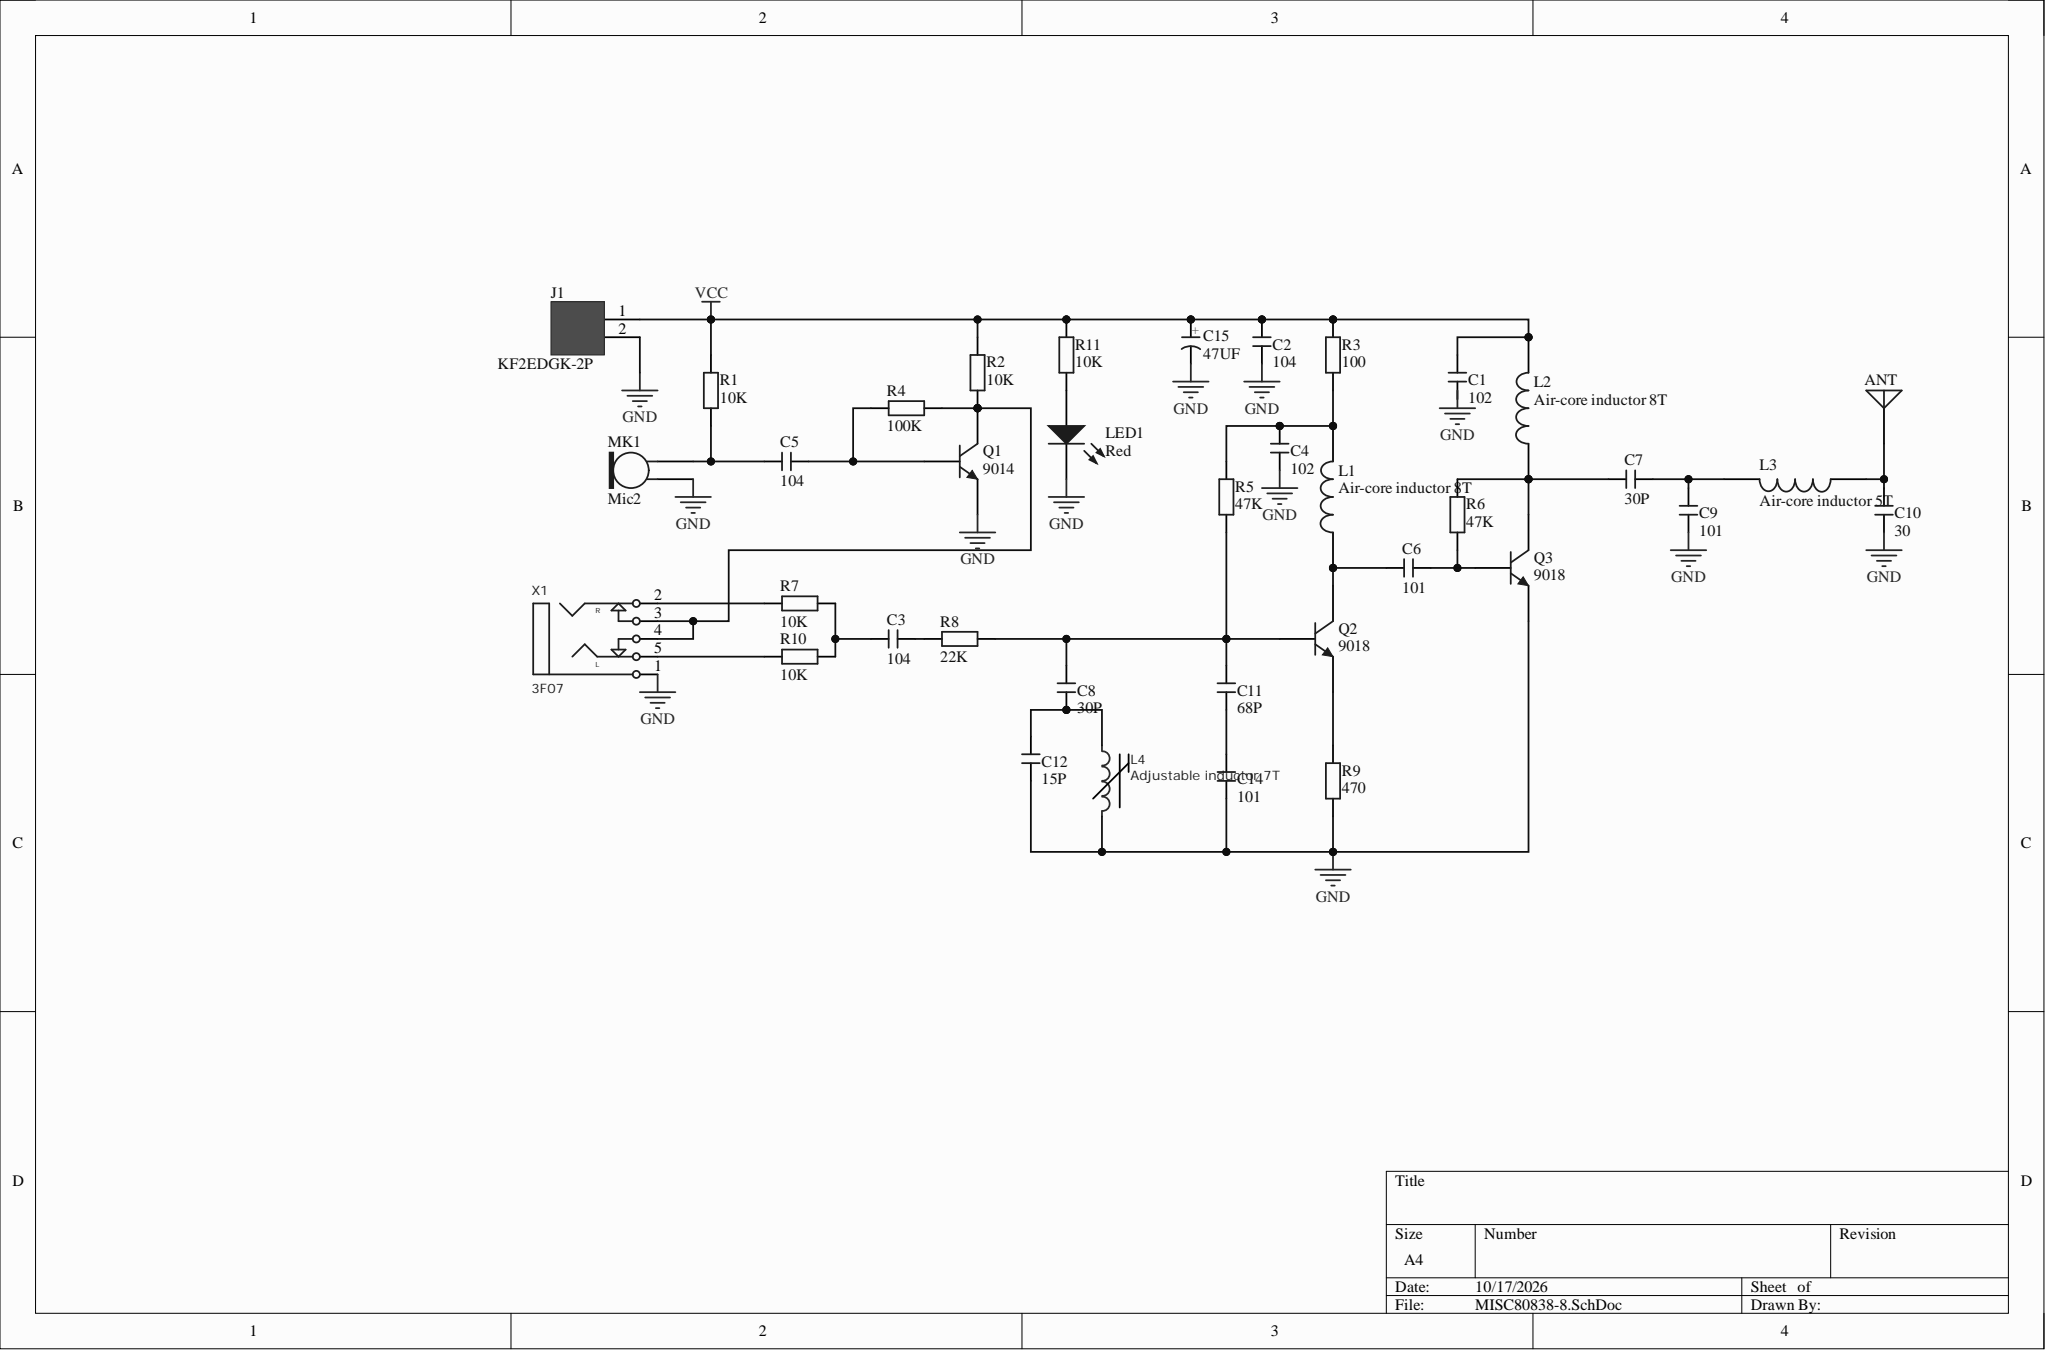Circuit board | Altium Designer | 37 parts | 20 nets
Bill of materials:
Comment,Description,Designator,Footprint,LibRef,Quantity
"Antenna","Generic Antenna","ANT","PIN1","Antenna","1"
"102","Ceramic capacitor","C1, C4","CC 1.8*3.6","CC","2"
"104","Ceramic capacitor","C2, C3, C5","CC 1.8*3.6","CC","3"
"101","Ceramic capacitor","C6, C9, C14","CC 1.8*3.6","CC","3"
"30P","Ceramic capacitor","C7, C8","CC 1.8*3.6","CC","2"
"30","Ceramic capacitor","C10","CC 1.8*3.6","CC","1"
"68P","Ceramic capacitor","C11","CC 1.8*3.6","CC","1"
"15P","Ceramic capacitor","C12","CC 1.8*3.6","CC","1"
"47UF","Through-hole solid-state capacitor","C15","CS 2.0*5*8 - C","CS","1"
"KF2EDGK-2P","","J1","KF2EDGK5.0-2P","KF2EDGK-2P","1"
"Air-core inductor 8T","Air-core inductor 8T","L1, L2","8T","INDUCTOR","2"
"Air-core inductor 5T","INDUCTOR","L3","5T","空心电感5T","1"
"Adjustable inductor 7T","Adjustable inductor 7T","L4","可调电感7T","IND_ADJ","1"
"Red","Through-hole 3mm LED","LED1","LED 3MM-B","LED-3MM","1"
"Mic2","Microphone","MK1","PIN2","Mic2","1"
"9014","NPN General Purpose Amplifier","Q1","TO-92A","2N3904","1"
"9018","NPN General Purpose Amplifier","Q2, Q3","TO-92A","2N3904","2"
"10K","Color-band resistor","R1, R2, R7, R10, R11","RS 1/4W","R-S","5"
"100","Color-band resistor","R3","RS 1/4W","R-S","1"
"100K","Color-band resistor","R4","RS 1/4W","R-S","1"
"47K","Color-band resistor","R5, R6","RS 1/4W","R-S","2"
"22K","Color-band resistor","R8","RS 1/4W","R-S","1"
"470","Color-band resistor","R9","RS 1/4W","R-S","1"
"3F07","","X1","3F07","3F07","1"
Netlist (Protel format):
[
ANT
PIN1
Antenna



]
[
C1
CC 1.8*3.6
102



]
[
C2
CC 1.8*3.6
104



]
[
C3
CC 1.8*3.6
104



]
[
C4
CC 1.8*3.6
102



]
[
C5
CC 1.8*3.6
104



]
[
C6
CC 1.8*3.6
101



]
[
C7
CC 1.8*3.6
30P



]
[
C8
CC 1.8*3.6
30P



]
[
C9
CC 1.8*3.6
101



]
[
C10
CC 1.8*3.6
30



]
[
C11
CC 1.8*3.6
68P



]
[
C12
CC 1.8*3.6
15P



]
[
C14
CC 1.8*3.6
101



]
[
C15
CS 2.0*5*8 - C
47UF



]
[
J1
KF2EDGK5.0-2P
KF2EDGK-2P



]
[
L1
8T
Air-core inductor 8T



]
[
L2
8T
Air-core inductor 8T



]
[
L3
5T
Air-core inductor 5T



]
[
L4
可调电感7T
Adjustable inductor 7T



]
[
LED1
LED 3MM-B
Red



]
[
MK1
PIN2
Mic2



]
[
Q1
TO-92A
9014



]
[
Q2
TO-92A
9018



]
[
Q3
TO-92A
9018



]
[
R1
RS 1/4W
10K



]
[
R2
RS 1/4W
10K



]
[
R3
RS 1/4W
100



]
[
R4
RS 1/4W
100K



]
[
R5
RS 1/4W
47K



]
[
R6
RS 1/4W
47K



]
[
R7
RS 1/4W
10K



]
[
R8
RS 1/4W
22K



]
[
R9
RS 1/4W
470



]
[
R10
RS 1/4W
10K



]
[
R11
RS 1/4W
10K



]
[
X1
3F07
3F07



]
(
VCC
C1-2
C2-2
C15-1
J1-1
L2-2
R1-2
R2-2
R3-1
R11-2
)
(
NetR10_1
R10-1
X1-5
)
(
NetR7_1
R7-1
X1-2
)
(
NetQ2_1
Q2-1
R9-1
)
(
NetQ1_3
Q1-3
R2-1
R4-1
X1-3
X1-4
)
(
NetLED1_1
LED1-1
R11-1
)
(
NetC11_2
C11-2
C14-1
)
(
NetC8_2
C8-2
C12-1
L4-2
)
(
NetC8_1
C8-1
C11-1
Q2-2
R5-2
R8-2
)
(
NetC7_2
C7-2
L2-1
Q3-3
R6-1
)
(
NetC7_1
C7-1
C9-1
L3-2
)
(
NetC6_2
C6-2
L1-1
Q2-3
)
(
NetC6_1
C6-1
Q3-2
R6-2
)
(
NetC5_2
C5-2
Q1-2
R4-2
)
(
NetC5_1
C5-1
MK1-2
R1-1
)
(
NetC4_2
C4-2
L1-2
R3-2
R5-1
)
(
NetC3_2
C3-2
R8-1
)
(
NetC3_1
C3-1
R7-2
R10-2
)
(
NetANT_1
ANT-1
C10-1
L3-1
)
(
GND
C2-1
C4-1
C9-2
C10-2
C12-2
C14-2
C15-2
J1-2
L4-1
LED1-2
MK1-1
Q1-1
Q3-1
R9-2
X1-1
)